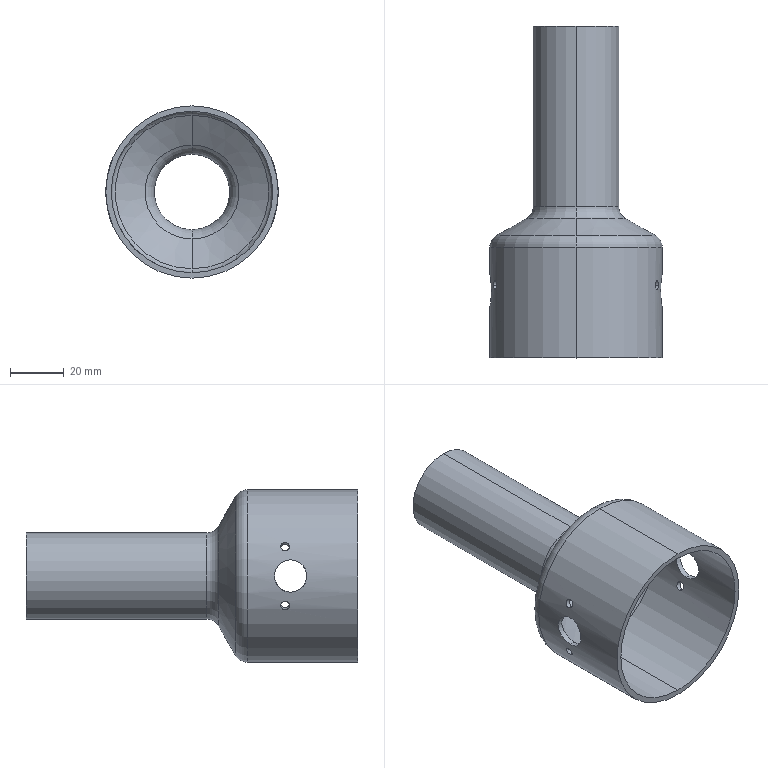Part | SolidWorks | features 3DProfileFeature 2, HoleWzd 2, Fillet 1, ICE 1, MirrorPattern 1, RefAxis 1, Revolution 1, Shell 1 | 1 solid | 34 faces | box 64 x 123.238 x 64 mm | volume 34756 mm3 | cylinder 20 | torus 8 | cone 4 | plane 2 | commonest cylinder face diameters 3.3 x8 12 x4 28 x2 32 x2 60 x2 64 x2